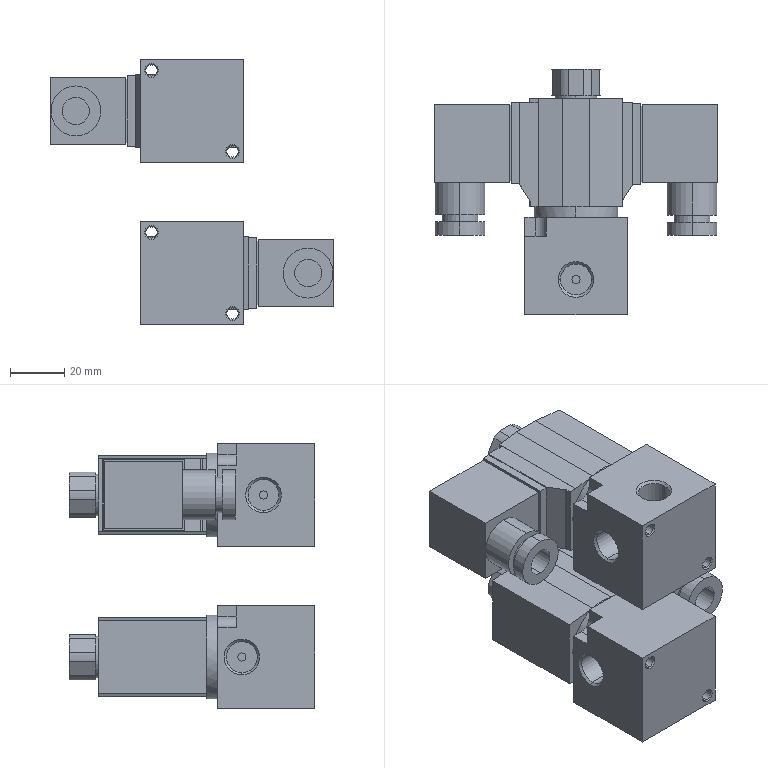Part | SolidWorks | 2 solids | 236 faces | box 105 x 90.9 x 98 mm | volume 242700 mm3 | plane 132 | cylinder 84 | cone 20 | commonest cylinder face diameters 3 x12 11.445 x12 18 x12 4.134 x8 4.2 x8 18.5 x8